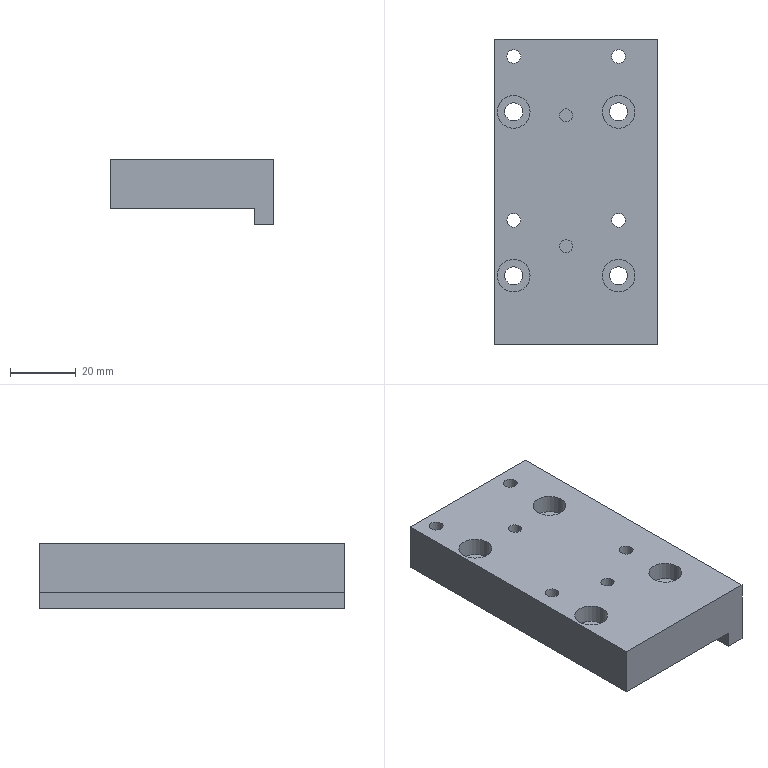Part | STEP file | SynoNew-0304-031 | 1 solid | 28 faces | box 50 x 93.3 x 20 mm | volume 69168 mm3 | cylinder 14 | plane 14 | commonest cylinder face diameters 4.2 x4 5.5 x4 10 x4 4 x2
STEP:
#1=CARTESIAN_POINT('',(-1.,-16.583,15.));
#2=VERTEX_POINT('',#1);
#3=CARTESIAN_POINT('',(-5.,-16.583,15.));
#4=VERTEX_POINT('',#3);
#5=CARTESIAN_POINT('',(-3.,-16.583,15.));
#6=DIRECTION('',(0.,0.,-1.));
#7=DIRECTION('',(1.,0.,0.));
#8=AXIS2_PLACEMENT_3D('',#5,#6,#7);
#9=CIRCLE('',#8,2.);
#10=EDGE_CURVE('',#2,#4,#9,.T.);
#11=ORIENTED_EDGE('',*,*,#10,.F.);
#12=CARTESIAN_POINT('',(-3.,-16.583,15.));
#13=DIRECTION('',(0.,0.,-1.));
#14=DIRECTION('',(1.,0.,0.));
#15=AXIS2_PLACEMENT_3D('',#12,#13,#14);
#16=CIRCLE('',#15,2.);
#17=EDGE_CURVE('',#4,#2,#16,.T.);
#18=ORIENTED_EDGE('',*,*,#17,.F.);
#19=CARTESIAN_POINT('',(-5.,-16.583,11.));
#20=VERTEX_POINT('',#19);
#21=CARTESIAN_POINT('',(-5.,-16.583,15.));
#22=DIRECTION('',(0.,0.,-1.));
#23=VECTOR('',#22,2.);
#24=LINE('',#21,#23);
#25=EDGE_CURVE('',#4,#20,#24,.T.);
#26=ORIENTED_EDGE('',*,*,#25,.T.);
#27=CARTESIAN_POINT('',(-1.,-16.583,11.));
#28=VERTEX_POINT('',#27);
#29=CARTESIAN_POINT('',(-3.,-16.583,11.));
#30=DIRECTION('',(0.,0.,-1.));
#31=DIRECTION('',(1.,0.,0.));
#32=AXIS2_PLACEMENT_3D('',#29,#30,#31);
#33=CIRCLE('',#32,2.);
#34=EDGE_CURVE('',#20,#28,#33,.T.);
#35=ORIENTED_EDGE('',*,*,#34,.T.);
#36=CARTESIAN_POINT('',(-3.,-16.583,11.));
#37=DIRECTION('',(0.,0.,-1.));
#38=DIRECTION('',(1.,0.,0.));
#39=AXIS2_PLACEMENT_3D('',#36,#37,#38);
#40=CIRCLE('',#39,2.);
#41=EDGE_CURVE('',#28,#20,#40,.T.);
#42=ORIENTED_EDGE('',*,*,#41,.T.);
#43=ORIENTED_EDGE('',*,*,#25,.F.);
#44=EDGE_LOOP('',(#11,#18,#26,#35,#42,#43));
#45=FACE_OUTER_BOUND('',#44,.T.);
#46=CARTESIAN_POINT('',(-3.,-16.583,15.));
#47=DIRECTION('',(0.,0.,-1.));
#48=DIRECTION('',(1.,0.,0.));
#49=AXIS2_PLACEMENT_3D('',#46,#47,#48);
#50=CYLINDRICAL_SURFACE('',#49,2.);
#51=ADVANCED_FACE('',(#45),#50,.F.);
#52=ORIENTED_EDGE('',*,*,#41,.F.);
#53=ORIENTED_EDGE('',*,*,#34,.F.);
#54=EDGE_LOOP('',(#52,#53));
#55=FACE_OUTER_BOUND('',#54,.T.);
#56=CARTESIAN_POINT('',(-3.,-16.583,11.));
#57=DIRECTION('',(0.,0.,1.));
#58=DIRECTION('',(1.,0.,0.));
#59=AXIS2_PLACEMENT_3D('',#56,#57,#58);
#60=PLANE('',#59);
#61=ADVANCED_FACE('',(#55),#60,.T.);
#62=CARTESIAN_POINT('',(-1.,23.35,15.));
#63=VERTEX_POINT('',#62);
#64=CARTESIAN_POINT('',(-5.,23.35,15.));
#65=VERTEX_POINT('',#64);
#66=CARTESIAN_POINT('',(-3.,23.35,15.));
#67=DIRECTION('',(0.,0.,-1.));
#68=DIRECTION('',(1.,0.,0.));
#69=AXIS2_PLACEMENT_3D('',#66,#67,#68);
#70=CIRCLE('',#69,2.);
#71=EDGE_CURVE('',#63,#65,#70,.T.);
#72=ORIENTED_EDGE('',*,*,#71,.F.);
#73=CARTESIAN_POINT('',(-3.,23.35,15.));
#74=DIRECTION('',(0.,0.,-1.));
#75=DIRECTION('',(1.,0.,0.));
#76=AXIS2_PLACEMENT_3D('',#73,#74,#75);
#77=CIRCLE('',#76,2.);
#78=EDGE_CURVE('',#65,#63,#77,.T.);
#79=ORIENTED_EDGE('',*,*,#78,.F.);
#80=CARTESIAN_POINT('',(-5.,23.35,11.));
#81=VERTEX_POINT('',#80);
#82=CARTESIAN_POINT('',(-5.,23.35,15.));
#83=DIRECTION('',(0.,0.,-1.));
#84=VECTOR('',#83,2.);
#85=LINE('',#82,#84);
#86=EDGE_CURVE('',#65,#81,#85,.T.);
#87=ORIENTED_EDGE('',*,*,#86,.T.);
#88=CARTESIAN_POINT('',(-1.,23.35,11.));
#89=VERTEX_POINT('',#88);
#90=CARTESIAN_POINT('',(-3.,23.35,11.));
#91=DIRECTION('',(0.,0.,-1.));
#92=DIRECTION('',(1.,0.,0.));
#93=AXIS2_PLACEMENT_3D('',#90,#91,#92);
#94=CIRCLE('',#93,2.);
#95=EDGE_CURVE('',#81,#89,#94,.T.);
#96=ORIENTED_EDGE('',*,*,#95,.T.);
#97=CARTESIAN_POINT('',(-3.,23.35,11.));
#98=DIRECTION('',(0.,0.,-1.));
#99=DIRECTION('',(1.,0.,0.));
#100=AXIS2_PLACEMENT_3D('',#97,#98,#99);
#101=CIRCLE('',#100,2.);
#102=EDGE_CURVE('',#89,#81,#101,.T.);
#103=ORIENTED_EDGE('',*,*,#102,.T.);
#104=ORIENTED_EDGE('',*,*,#86,.F.);
#105=EDGE_LOOP('',(#72,#79,#87,#96,#103,#104));
#106=FACE_OUTER_BOUND('',#105,.T.);
#107=CARTESIAN_POINT('',(-3.,23.35,15.));
#108=DIRECTION('',(0.,0.,-1.));
#109=DIRECTION('',(1.,0.,0.));
#110=AXIS2_PLACEMENT_3D('',#107,#108,#109);
#111=CYLINDRICAL_SURFACE('',#110,2.);
#112=ADVANCED_FACE('',(#106),#111,.F.);
#113=ORIENTED_EDGE('',*,*,#102,.F.);
#114=ORIENTED_EDGE('',*,*,#95,.F.);
#115=EDGE_LOOP('',(#113,#114));
#116=FACE_OUTER_BOUND('',#115,.T.);
#117=CARTESIAN_POINT('',(-3.,23.35,11.));
#118=DIRECTION('',(0.,0.,1.));
#119=DIRECTION('',(1.,0.,0.));
#120=AXIS2_PLACEMENT_3D('',#117,#118,#119);
#121=PLANE('',#120);
#122=ADVANCED_FACE('',(#116),#121,.T.);
#123=CARTESIAN_POINT('',(15.1,-8.65,15.));
#124=VERTEX_POINT('',#123);
#125=CARTESIAN_POINT('',(10.9,-8.65,15.));
#126=VERTEX_POINT('',#125);
#127=CARTESIAN_POINT('',(13.,-8.65,15.));
#128=DIRECTION('',(0.,0.,-1.));
#129=DIRECTION('',(1.,0.,0.));
#130=AXIS2_PLACEMENT_3D('',#127,#128,#129);
#131=CIRCLE('',#130,2.1);
#132=EDGE_CURVE('',#124,#126,#131,.T.);
#133=ORIENTED_EDGE('',*,*,#132,.F.);
#134=CARTESIAN_POINT('',(13.,-8.65,15.));
#135=DIRECTION('',(0.,0.,-1.));
#136=DIRECTION('',(1.,0.,0.));
#137=AXIS2_PLACEMENT_3D('',#134,#135,#136);
#138=CIRCLE('',#137,2.1);
#139=EDGE_CURVE('',#126,#124,#138,.T.);
#140=ORIENTED_EDGE('',*,*,#139,.F.);
#141=CARTESIAN_POINT('',(10.9,-8.65,0.));
#142=VERTEX_POINT('',#141);
#143=CARTESIAN_POINT('',(10.9,-8.65,-92.726));
#144=DIRECTION('',(0.,0.,-1.));
#145=VECTOR('',#144,2.1);
#146=LINE('',#143,#145);
#147=EDGE_CURVE('',#126,#142,#146,.T.);
#148=ORIENTED_EDGE('',*,*,#147,.T.);
#149=CARTESIAN_POINT('',(13.,-8.65,0.));
#150=DIRECTION('',(0.,0.,1.));
#151=DIRECTION('',(1.,0.,0.));
#152=AXIS2_PLACEMENT_3D('',#149,#150,#151);
#153=CIRCLE('',#152,2.1);
#154=EDGE_CURVE('',#142,#142,#153,.T.);
#155=ORIENTED_EDGE('',*,*,#154,.F.);
#156=ORIENTED_EDGE('',*,*,#147,.F.);
#157=EDGE_LOOP('',(#133,#140,#148,#155,#156));
#158=FACE_OUTER_BOUND('',#157,.T.);
#159=CARTESIAN_POINT('',(13.,-8.65,-92.726));
#160=DIRECTION('',(0.,0.,1.));
#161=DIRECTION('',(1.,0.,0.));
#162=AXIS2_PLACEMENT_3D('',#159,#160,#161);
#163=CYLINDRICAL_SURFACE('',#162,2.1);
#164=ADVANCED_FACE('',(#158),#163,.F.);
#165=CARTESIAN_POINT('',(-16.9,41.35,15.));
#166=VERTEX_POINT('',#165);
#167=CARTESIAN_POINT('',(-21.1,41.35,15.));
#168=VERTEX_POINT('',#167);
#169=CARTESIAN_POINT('',(-19.,41.35,15.));
#170=DIRECTION('',(0.,0.,-1.));
#171=DIRECTION('',(1.,0.,0.));
#172=AXIS2_PLACEMENT_3D('',#169,#170,#171);
#173=CIRCLE('',#172,2.1);
#174=EDGE_CURVE('',#166,#168,#173,.T.);
#175=ORIENTED_EDGE('',*,*,#174,.F.);
#176=CARTESIAN_POINT('',(-19.,41.35,15.));
#177=DIRECTION('',(0.,0.,-1.));
#178=DIRECTION('',(1.,0.,0.));
#179=AXIS2_PLACEMENT_3D('',#176,#177,#178);
#180=CIRCLE('',#179,2.1);
#181=EDGE_CURVE('',#168,#166,#180,.T.);
#182=ORIENTED_EDGE('',*,*,#181,.F.);
#183=CARTESIAN_POINT('',(-21.1,41.35,0.));
#184=VERTEX_POINT('',#183);
#185=CARTESIAN_POINT('',(-21.1,41.35,-92.726));
#186=DIRECTION('',(0.,0.,-1.));
#187=VECTOR('',#186,2.1);
#188=LINE('',#185,#187);
#189=EDGE_CURVE('',#168,#184,#188,.T.);
#190=ORIENTED_EDGE('',*,*,#189,.T.);
#191=CARTESIAN_POINT('',(-19.,41.35,0.));
#192=DIRECTION('',(0.,0.,1.));
#193=DIRECTION('',(1.,0.,0.));
#194=AXIS2_PLACEMENT_3D('',#191,#192,#193);
#195=CIRCLE('',#194,2.1);
#196=EDGE_CURVE('',#184,#184,#195,.T.);
#197=ORIENTED_EDGE('',*,*,#196,.F.);
#198=ORIENTED_EDGE('',*,*,#189,.F.);
#199=EDGE_LOOP('',(#175,#182,#190,#197,#198));
#200=FACE_OUTER_BOUND('',#199,.T.);
#201=CARTESIAN_POINT('',(-19.,41.35,-92.726));
#202=DIRECTION('',(0.,0.,1.));
#203=DIRECTION('',(1.,0.,0.));
#204=AXIS2_PLACEMENT_3D('',#201,#202,#203);
#205=CYLINDRICAL_SURFACE('',#204,2.1);
#206=ADVANCED_FACE('',(#200),#205,.F.);
#207=CARTESIAN_POINT('',(15.1,41.35,15.));
#208=VERTEX_POINT('',#207);
#209=CARTESIAN_POINT('',(10.9,41.35,15.));
#210=VERTEX_POINT('',#209);
#211=CARTESIAN_POINT('',(13.,41.35,15.));
#212=DIRECTION('',(0.,0.,-1.));
#213=DIRECTION('',(1.,0.,0.));
#214=AXIS2_PLACEMENT_3D('',#211,#212,#213);
#215=CIRCLE('',#214,2.1);
#216=EDGE_CURVE('',#208,#210,#215,.T.);
#217=ORIENTED_EDGE('',*,*,#216,.F.);
#218=CARTESIAN_POINT('',(13.,41.35,15.));
#219=DIRECTION('',(0.,0.,-1.));
#220=DIRECTION('',(1.,0.,0.));
#221=AXIS2_PLACEMENT_3D('',#218,#219,#220);
#222=CIRCLE('',#221,2.1);
#223=EDGE_CURVE('',#210,#208,#222,.T.);
#224=ORIENTED_EDGE('',*,*,#223,.F.);
#225=CARTESIAN_POINT('',(10.9,41.35,0.));
#226=VERTEX_POINT('',#225);
#227=CARTESIAN_POINT('',(10.9,41.35,-92.726));
#228=DIRECTION('',(0.,0.,-1.));
#229=VECTOR('',#228,2.1);
#230=LINE('',#227,#229);
#231=EDGE_CURVE('',#210,#226,#230,.T.);
#232=ORIENTED_EDGE('',*,*,#231,.T.);
#233=CARTESIAN_POINT('',(13.,41.35,0.));
#234=DIRECTION('',(0.,0.,1.));
#235=DIRECTION('',(1.,0.,0.));
#236=AXIS2_PLACEMENT_3D('',#233,#234,#235);
#237=CIRCLE('',#236,2.1);
#238=EDGE_CURVE('',#226,#226,#237,.T.);
#239=ORIENTED_EDGE('',*,*,#238,.F.);
#240=ORIENTED_EDGE('',*,*,#231,.F.);
#241=EDGE_LOOP('',(#217,#224,#232,#239,#240));
#242=FACE_OUTER_BOUND('',#241,.T.);
#243=CARTESIAN_POINT('',(13.,41.35,-92.726));
#244=DIRECTION('',(0.,0.,1.));
#245=DIRECTION('',(1.,0.,0.));
#246=AXIS2_PLACEMENT_3D('',#243,#244,#245);
#247=CYLINDRICAL_SURFACE('',#246,2.1);
#248=ADVANCED_FACE('',(#242),#247,.F.);
#249=CARTESIAN_POINT('',(-16.9,-8.65,15.));
#250=VERTEX_POINT('',#249);
#251=CARTESIAN_POINT('',(-21.1,-8.65,15.));
#252=VERTEX_POINT('',#251);
#253=CARTESIAN_POINT('',(-19.,-8.65,15.));
#254=DIRECTION('',(0.,0.,-1.));
#255=DIRECTION('',(1.,0.,0.));
#256=AXIS2_PLACEMENT_3D('',#253,#254,#255);
#257=CIRCLE('',#256,2.1);
#258=EDGE_CURVE('',#250,#252,#257,.T.);
#259=ORIENTED_EDGE('',*,*,#258,.F.);
#260=CARTESIAN_POINT('',(-19.,-8.65,15.));
#261=DIRECTION('',(0.,0.,-1.));
#262=DIRECTION('',(1.,0.,0.));
#263=AXIS2_PLACEMENT_3D('',#260,#261,#262);
#264=CIRCLE('',#263,2.1);
#265=EDGE_CURVE('',#252,#250,#264,.T.);
#266=ORIENTED_EDGE('',*,*,#265,.F.);
#267=CARTESIAN_POINT('',(-21.1,-8.65,0.));
#268=VERTEX_POINT('',#267);
#269=CARTESIAN_POINT('',(-21.1,-8.65,-92.726));
#270=DIRECTION('',(0.,0.,-1.));
#271=VECTOR('',#270,2.1);
#272=LINE('',#269,#271);
#273=EDGE_CURVE('',#252,#268,#272,.T.);
#274=ORIENTED_EDGE('',*,*,#273,.T.);
#275=CARTESIAN_POINT('',(-19.,-8.65,0.));
#276=DIRECTION('',(0.,0.,1.));
#277=DIRECTION('',(1.,0.,0.));
#278=AXIS2_PLACEMENT_3D('',#275,#276,#277);
#279=CIRCLE('',#278,2.1);
#280=EDGE_CURVE('',#268,#268,#279,.T.);
#281=ORIENTED_EDGE('',*,*,#280,.F.);
#282=ORIENTED_EDGE('',*,*,#273,.F.);
#283=EDGE_LOOP('',(#259,#266,#274,#281,#282));
#284=FACE_OUTER_BOUND('',#283,.T.);
#285=CARTESIAN_POINT('',(-19.,-8.65,-92.726));
#286=DIRECTION('',(0.,0.,1.));
#287=DIRECTION('',(1.,0.,0.));
#288=AXIS2_PLACEMENT_3D('',#285,#286,#287);
#289=CYLINDRICAL_SURFACE('',#288,2.1);
#290=ADVANCED_FACE('',(#284),#289,.F.);
#291=CARTESIAN_POINT('',(18.,-25.55,9.3));
#292=VERTEX_POINT('',#291);
#293=CARTESIAN_POINT('',(8.,-25.55,9.3));
#294=VERTEX_POINT('',#293);
#295=CARTESIAN_POINT('',(13.,-25.55,9.3));
#296=DIRECTION('',(0.,0.,1.));
#297=DIRECTION('',(1.,0.,0.));
#298=AXIS2_PLACEMENT_3D('',#295,#296,#297);
#299=CIRCLE('',#298,5.);
#300=EDGE_CURVE('',#292,#294,#299,.T.);
#301=ORIENTED_EDGE('',*,*,#300,.T.);
#302=CARTESIAN_POINT('',(13.,-25.55,9.3));
#303=DIRECTION('',(0.,0.,1.));
#304=DIRECTION('',(1.,0.,0.));
#305=AXIS2_PLACEMENT_3D('',#302,#303,#304);
#306=CIRCLE('',#305,5.);
#307=EDGE_CURVE('',#294,#292,#306,.T.);
#308=ORIENTED_EDGE('',*,*,#307,.T.);
#309=EDGE_LOOP('',(#301,#308));
#310=FACE_OUTER_BOUND('',#309,.T.);
#311=CARTESIAN_POINT('',(10.25,-25.55,9.3));
#312=VERTEX_POINT('',#311);
#313=CARTESIAN_POINT('',(13.,-25.55,9.3));
#314=DIRECTION('',(0.,0.,1.));
#315=DIRECTION('',(1.,0.,0.));
#316=AXIS2_PLACEMENT_3D('',#313,#314,#315);
#317=CIRCLE('',#316,2.75);
#318=EDGE_CURVE('',#312,#312,#317,.T.);
#319=ORIENTED_EDGE('',*,*,#318,.F.);
#320=EDGE_LOOP('',(#319));
#321=FACE_BOUND('',#320,.T.);
#322=CARTESIAN_POINT('',(13.,-25.55,9.3));
#323=DIRECTION('',(0.,0.,1.));
#324=DIRECTION('',(1.,0.,0.));
#325=AXIS2_PLACEMENT_3D('',#322,#323,#324);
#326=PLANE('',#325);
#327=ADVANCED_FACE('',(#310,#321),#326,.T.);
#328=CARTESIAN_POINT('',(18.,-25.55,15.));
#329=VERTEX_POINT('',#328);
#330=CARTESIAN_POINT('',(8.,-25.55,15.));
#331=VERTEX_POINT('',#330);
#332=CARTESIAN_POINT('',(13.,-25.55,15.));
#333=DIRECTION('',(0.,0.,-1.));
#334=DIRECTION('',(1.,0.,0.));
#335=AXIS2_PLACEMENT_3D('',#332,#333,#334);
#336=CIRCLE('',#335,5.);
#337=EDGE_CURVE('',#329,#331,#336,.T.);
#338=ORIENTED_EDGE('',*,*,#337,.F.);
#339=CARTESIAN_POINT('',(13.,-25.55,15.));
#340=DIRECTION('',(0.,0.,-1.));
#341=DIRECTION('',(1.,0.,0.));
#342=AXIS2_PLACEMENT_3D('',#339,#340,#341);
#343=CIRCLE('',#342,5.);
#344=EDGE_CURVE('',#331,#329,#343,.T.);
#345=ORIENTED_EDGE('',*,*,#344,.F.);
#346=CARTESIAN_POINT('',(8.,-25.55,12.15));
#347=DIRECTION('',(0.,0.,-1.));
#348=VECTOR('',#347,5.);
#349=LINE('',#346,#348);
#350=EDGE_CURVE('',#331,#294,#349,.T.);
#351=ORIENTED_EDGE('',*,*,#350,.T.);
#352=ORIENTED_EDGE('',*,*,#300,.F.);
#353=ORIENTED_EDGE('',*,*,#307,.F.);
#354=ORIENTED_EDGE('',*,*,#350,.F.);
#355=EDGE_LOOP('',(#338,#345,#351,#352,#353,#354));
#356=FACE_OUTER_BOUND('',#355,.T.);
#357=CARTESIAN_POINT('',(13.,-25.55,12.15));
#358=DIRECTION('',(0.,0.,1.));
#359=DIRECTION('',(1.,0.,0.));
#360=AXIS2_PLACEMENT_3D('',#357,#358,#359);
#361=CYLINDRICAL_SURFACE('',#360,5.);
#362=ADVANCED_FACE('',(#356),#361,.F.);
#363=ORIENTED_EDGE('',*,*,#318,.T.);
#364=CARTESIAN_POINT('',(10.25,-25.55,0.));
#365=VERTEX_POINT('',#364);
#366=CARTESIAN_POINT('',(10.25,-25.55,-92.726));
#367=DIRECTION('',(0.,0.,-1.));
#368=VECTOR('',#367,2.75);
#369=LINE('',#366,#368);
#370=EDGE_CURVE('',#312,#365,#369,.T.);
#371=ORIENTED_EDGE('',*,*,#370,.T.);
#372=CARTESIAN_POINT('',(13.,-25.55,0.));
#373=DIRECTION('',(0.,0.,1.));
#374=DIRECTION('',(1.,0.,0.));
#375=AXIS2_PLACEMENT_3D('',#372,#373,#374);
#376=CIRCLE('',#375,2.75);
#377=EDGE_CURVE('',#365,#365,#376,.T.);
#378=ORIENTED_EDGE('',*,*,#377,.F.);
#379=ORIENTED_EDGE('',*,*,#370,.F.);
#380=EDGE_LOOP('',(#363,#371,#378,#379));
#381=FACE_OUTER_BOUND('',#380,.T.);
#382=CARTESIAN_POINT('',(13.,-25.55,-92.726));
#383=DIRECTION('',(0.,0.,1.));
#384=DIRECTION('',(1.,0.,0.));
#385=AXIS2_PLACEMENT_3D('',#382,#383,#384);
#386=CYLINDRICAL_SURFACE('',#385,2.75);
#387=ADVANCED_FACE('',(#381),#386,.F.);
#388=CARTESIAN_POINT('',(18.,24.45,9.3));
#389=VERTEX_POINT('',#388);
#390=CARTESIAN_POINT('',(8.,24.45,9.3));
#391=VERTEX_POINT('',#390);
#392=CARTESIAN_POINT('',(13.,24.45,9.3));
#393=DIRECTION('',(0.,0.,1.));
#394=DIRECTION('',(1.,0.,0.));
#395=AXIS2_PLACEMENT_3D('',#392,#393,#394);
#396=CIRCLE('',#395,5.);
#397=EDGE_CURVE('',#389,#391,#396,.T.);
#398=ORIENTED_EDGE('',*,*,#397,.T.);
#399=CARTESIAN_POINT('',(13.,24.45,9.3));
#400=DIRECTION('',(0.,0.,1.));
#401=DIRECTION('',(1.,0.,0.));
#402=AXIS2_PLACEMENT_3D('',#399,#400,#401);
#403=CIRCLE('',#402,5.);
#404=EDGE_CURVE('',#391,#389,#403,.T.);
#405=ORIENTED_EDGE('',*,*,#404,.T.);
#406=EDGE_LOOP('',(#398,#405));
#407=FACE_OUTER_BOUND('',#406,.T.);
#408=CARTESIAN_POINT('',(10.25,24.45,9.3));
#409=VERTEX_POINT('',#408);
#410=CARTESIAN_POINT('',(13.,24.45,9.3));
#411=DIRECTION('',(0.,0.,1.));
#412=DIRECTION('',(1.,0.,0.));
#413=AXIS2_PLACEMENT_3D('',#410,#411,#412);
#414=CIRCLE('',#413,2.75);
#415=EDGE_CURVE('',#409,#409,#414,.T.);
#416=ORIENTED_EDGE('',*,*,#415,.F.);
#417=EDGE_LOOP('',(#416));
#418=FACE_BOUND('',#417,.T.);
#419=CARTESIAN_POINT('',(13.,24.45,9.3));
#420=DIRECTION('',(0.,0.,1.));
#421=DIRECTION('',(1.,0.,0.));
#422=AXIS2_PLACEMENT_3D('',#419,#420,#421);
#423=PLANE('',#422);
#424=ADVANCED_FACE('',(#407,#418),#423,.T.);
#425=CARTESIAN_POINT('',(18.,24.45,15.));
#426=VERTEX_POINT('',#425);
#427=CARTESIAN_POINT('',(8.,24.45,15.));
#428=VERTEX_POINT('',#427);
#429=CARTESIAN_POINT('',(13.,24.45,15.));
#430=DIRECTION('',(0.,0.,-1.));
#431=DIRECTION('',(1.,0.,0.));
#432=AXIS2_PLACEMENT_3D('',#429,#430,#431);
#433=CIRCLE('',#432,5.);
#434=EDGE_CURVE('',#426,#428,#433,.T.);
#435=ORIENTED_EDGE('',*,*,#434,.F.);
#436=CARTESIAN_POINT('',(13.,24.45,15.));
#437=DIRECTION('',(0.,0.,-1.));
#438=DIRECTION('',(1.,0.,0.));
#439=AXIS2_PLACEMENT_3D('',#436,#437,#438);
#440=CIRCLE('',#439,5.);
#441=EDGE_CURVE('',#428,#426,#440,.T.);
#442=ORIENTED_EDGE('',*,*,#441,.F.);
#443=CARTESIAN_POINT('',(8.,24.45,12.15));
#444=DIRECTION('',(0.,0.,-1.));
#445=VECTOR('',#444,5.);
#446=LINE('',#443,#445);
#447=EDGE_CURVE('',#428,#391,#446,.T.);
#448=ORIENTED_EDGE('',*,*,#447,.T.);
#449=ORIENTED_EDGE('',*,*,#397,.F.);
#450=ORIENTED_EDGE('',*,*,#404,.F.);
#451=ORIENTED_EDGE('',*,*,#447,.F.);
#452=EDGE_LOOP('',(#435,#442,#448,#449,#450,#451));
#453=FACE_OUTER_BOUND('',#452,.T.);
#454=CARTESIAN_POINT('',(13.,24.45,12.15));
#455=DIRECTION('',(0.,0.,1.));
#456=DIRECTION('',(1.,0.,0.));
#457=AXIS2_PLACEMENT_3D('',#454,#455,#456);
#458=CYLINDRICAL_SURFACE('',#457,5.);
#459=ADVANCED_FACE('',(#453),#458,.F.);
#460=ORIENTED_EDGE('',*,*,#415,.T.);
#461=CARTESIAN_POINT('',(10.25,24.45,0.));
#462=VERTEX_POINT('',#461);
#463=CARTESIAN_POINT('',(10.25,24.45,-92.726));
#464=DIRECTION('',(0.,0.,-1.));
#465=VECTOR('',#464,2.75);
#466=LINE('',#463,#465);
#467=EDGE_CURVE('',#409,#462,#466,.T.);
#468=ORIENTED_EDGE('',*,*,#467,.T.);
#469=CARTESIAN_POINT('',(13.,24.45,0.));
#470=DIRECTION('',(0.,0.,1.));
#471=DIRECTION('',(1.,0.,0.));
#472=AXIS2_PLACEMENT_3D('',#469,#470,#471);
#473=CIRCLE('',#472,2.75);
#474=EDGE_CURVE('',#462,#462,#473,.T.);
#475=ORIENTED_EDGE('',*,*,#474,.F.);
#476=ORIENTED_EDGE('',*,*,#467,.F.);
#477=EDGE_LOOP('',(#460,#468,#475,#476));
#478=FACE_OUTER_BOUND('',#477,.T.);
#479=CARTESIAN_POINT('',(13.,24.45,-92.726));
#480=DIRECTION('',(0.,0.,1.));
#481=DIRECTION('',(1.,0.,0.));
#482=AXIS2_PLACEMENT_3D('',#479,#480,#481);
#483=CYLINDRICAL_SURFACE('',#482,2.75);
#484=ADVANCED_FACE('',(#478),#483,.F.);
#485=CARTESIAN_POINT('',(-14.,24.45,9.3));
#486=VERTEX_POINT('',#485);
#487=CARTESIAN_POINT('',(-24.,24.45,9.3));
#488=VERTEX_POINT('',#487);
#489=CARTESIAN_POINT('',(-19.,24.45,9.3));
#490=DIRECTION('',(0.,0.,1.));
#491=DIRECTION('',(1.,0.,0.));
#492=AXIS2_PLACEMENT_3D('',#489,#490,#491);
#493=CIRCLE('',#492,5.);
#494=EDGE_CURVE('',#486,#488,#493,.T.);
#495=ORIENTED_EDGE('',*,*,#494,.T.);
#496=CARTESIAN_POINT('',(-19.,24.45,9.3));
#497=DIRECTION('',(0.,0.,1.));
#498=DIRECTION('',(1.,0.,0.));
#499=AXIS2_PLACEMENT_3D('',#496,#497,#498);
#500=CIRCLE('',#499,5.);
#501=EDGE_CURVE('',#488,#486,#500,.T.);
#502=ORIENTED_EDGE('',*,*,#501,.T.);
#503=EDGE_LOOP('',(#495,#502));
#504=FACE_OUTER_BOUND('',#503,.T.);
#505=CARTESIAN_POINT('',(-21.75,24.45,9.3));
#506=VERTEX_POINT('',#505);
#507=CARTESIAN_POINT('',(-19.,24.45,9.3));
#508=DIRECTION('',(0.,0.,1.));
#509=DIRECTION('',(1.,0.,0.));
#510=AXIS2_PLACEMENT_3D('',#507,#508,#509);
#511=CIRCLE('',#510,2.75);
#512=EDGE_CURVE('',#506,#506,#511,.T.);
#513=ORIENTED_EDGE('',*,*,#512,.F.);
#514=EDGE_LOOP('',(#513));
#515=FACE_BOUND('',#514,.T.);
#516=CARTESIAN_POINT('',(-19.,24.45,9.3));
#517=DIRECTION('',(0.,0.,1.));
#518=DIRECTION('',(1.,0.,0.));
#519=AXIS2_PLACEMENT_3D('',#516,#517,#518);
#520=PLANE('',#519);
#521=ADVANCED_FACE('',(#504,#515),#520,.T.);
#522=CARTESIAN_POINT('',(-14.,24.45,15.));
#523=VERTEX_POINT('',#522);
#524=CARTESIAN_POINT('',(-24.,24.45,15.));
#525=VERTEX_POINT('',#524);
#526=CARTESIAN_POINT('',(-19.,24.45,15.));
#527=DIRECTION('',(0.,0.,-1.));
#528=DIRECTION('',(1.,0.,0.));
#529=AXIS2_PLACEMENT_3D('',#526,#527,#528);
#530=CIRCLE('',#529,5.);
#531=EDGE_CURVE('',#523,#525,#530,.T.);
#532=ORIENTED_EDGE('',*,*,#531,.F.);
#533=CARTESIAN_POINT('',(-19.,24.45,15.));
#534=DIRECTION('',(0.,0.,-1.));
#535=DIRECTION('',(1.,0.,0.));
#536=AXIS2_PLACEMENT_3D('',#533,#534,#535);
#537=CIRCLE('',#536,5.);
#538=EDGE_CURVE('',#525,#523,#537,.T.);
#539=ORIENTED_EDGE('',*,*,#538,.F.);
#540=CARTESIAN_POINT('',(-24.,24.45,12.15));
#541=DIRECTION('',(0.,0.,-1.));
#542=VECTOR('',#541,5.);
#543=LINE('',#540,#542);
#544=EDGE_CURVE('',#525,#488,#543,.T.);
#545=ORIENTED_EDGE('',*,*,#544,.T.);
#546=ORIENTED_EDGE('',*,*,#494,.F.);
#547=ORIENTED_EDGE('',*,*,#501,.F.);
#548=ORIENTED_EDGE('',*,*,#544,.F.);
#549=EDGE_LOOP('',(#532,#539,#545,#546,#547,#548));
#550=FACE_OUTER_BOUND('',#549,.T.);
#551=CARTESIAN_POINT('',(-19.,24.45,12.15));
#552=DIRECTION('',(0.,0.,1.));
#553=DIRECTION('',(1.,0.,0.));
#554=AXIS2_PLACEMENT_3D('',#551,#552,#553);
#555=CYLINDRICAL_SURFACE('',#554,5.);
#556=ADVANCED_FACE('',(#550),#555,.F.);
#557=ORIENTED_EDGE('',*,*,#512,.T.);
#558=CARTESIAN_POINT('',(-21.75,24.45,0.));
#559=VERTEX_POINT('',#558);
#560=CARTESIAN_POINT('',(-21.75,24.45,-92.726));
#561=DIRECTION('',(0.,0.,-1.));
#562=VECTOR('',#561,2.75);
#563=LINE('',#560,#562);
#564=EDGE_CURVE('',#506,#559,#563,.T.);
#565=ORIENTED_EDGE('',*,*,#564,.T.);
#566=CARTESIAN_POINT('',(-19.,24.45,0.));
#567=DIRECTION('',(0.,0.,1.));
#568=DIRECTION('',(1.,0.,0.));
#569=AXIS2_PLACEMENT_3D('',#566,#567,#568);
#570=CIRCLE('',#569,2.75);
#571=EDGE_CURVE('',#559,#559,#570,.T.);
#572=ORIENTED_EDGE('',*,*,#571,.F.);
#573=ORIENTED_EDGE('',*,*,#564,.F.);
#574=EDGE_LOOP('',(#557,#565,#572,#573));
#575=FACE_OUTER_BOUND('',#574,.T.);
#576=CARTESIAN_POINT('',(-19.,24.45,-92.726));
#577=DIRECTION('',(0.,0.,1.));
#578=DIRECTION('',(1.,0.,0.));
#579=AXIS2_PLACEMENT_3D('',#576,#577,#578);
#580=CYLINDRICAL_SURFACE('',#579,2.75);
#581=ADVANCED_FACE('',(#575),#580,.F.);
#582=CARTESIAN_POINT('',(-14.,-25.55,9.3));
#583=VERTEX_POINT('',#582);
#584=CARTESIAN_POINT('',(-24.,-25.55,9.3));
#585=VERTEX_POINT('',#584);
#586=CARTESIAN_POINT('',(-19.,-25.55,9.3));
#587=DIRECTION('',(0.,0.,1.));
#588=DIRECTION('',(1.,0.,0.));
#589=AXIS2_PLACEMENT_3D('',#586,#587,#588);
#590=CIRCLE('',#589,5.);
#591=EDGE_CURVE('',#583,#585,#590,.T.);
#592=ORIENTED_EDGE('',*,*,#591,.T.);
#593=CARTESIAN_POINT('',(-19.,-25.55,9.3));
#594=DIRECTION('',(0.,0.,1.));
#595=DIRECTION('',(1.,0.,0.));
#596=AXIS2_PLACEMENT_3D('',#593,#594,#595);
#597=CIRCLE('',#596,5.);
#598=EDGE_CURVE('',#585,#583,#597,.T.);
#599=ORIENTED_EDGE('',*,*,#598,.T.);
#600=EDGE_LOOP('',(#592,#599));
#601=FACE_OUTER_BOUND('',#600,.T.);
#602=CARTESIAN_POINT('',(-21.75,-25.55,9.3));
#603=VERTEX_POINT('',#602);
#604=CARTESIAN_POINT('',(-19.,-25.55,9.3));
#605=DIRECTION('',(0.,0.,1.));
#606=DIRECTION('',(1.,0.,0.));
#607=AXIS2_PLACEMENT_3D('',#604,#605,#606);
#608=CIRCLE('',#607,2.75);
#609=EDGE_CURVE('',#603,#603,#608,.T.);
#610=ORIENTED_EDGE('',*,*,#609,.F.);
#611=EDGE_LOOP('',(#610));
#612=FACE_BOUND('',#611,.T.);
#613=CARTESIAN_POINT('',(-19.,-25.55,9.3));
#614=DIRECTION('',(0.,0.,1.));
#615=DIRECTION('',(1.,0.,0.));
#616=AXIS2_PLACEMENT_3D('',#613,#614,#615);
#617=PLANE('',#616);
#618=ADVANCED_FACE('',(#601,#612),#617,.T.);
#619=CARTESIAN_POINT('',(-14.,-25.55,15.));
#620=VERTEX_POINT('',#619);
#621=CARTESIAN_POINT('',(-24.,-25.55,15.));
#622=VERTEX_POINT('',#621);
#623=CARTESIAN_POINT('',(-19.,-25.55,15.));
#624=DIRECTION('',(0.,0.,-1.));
#625=DIRECTION('',(1.,0.,0.));
#626=AXIS2_PLACEMENT_3D('',#623,#624,#625);
#627=CIRCLE('',#626,5.);
#628=EDGE_CURVE('',#620,#622,#627,.T.);
#629=ORIENTED_EDGE('',*,*,#628,.F.);
#630=CARTESIAN_POINT('',(-19.,-25.55,15.));
#631=DIRECTION('',(0.,0.,-1.));
#632=DIRECTION('',(1.,0.,0.));
#633=AXIS2_PLACEMENT_3D('',#630,#631,#632);
#634=CIRCLE('',#633,5.);
#635=EDGE_CURVE('',#622,#620,#634,.T.);
#636=ORIENTED_EDGE('',*,*,#635,.F.);
#637=CARTESIAN_POINT('',(-24.,-25.55,12.15));
#638=DIRECTION('',(0.,0.,-1.));
#639=VECTOR('',#638,5.);
#640=LINE('',#637,#639);
#641=EDGE_CURVE('',#622,#585,#640,.T.);
#642=ORIENTED_EDGE('',*,*,#641,.T.);
#643=ORIENTED_EDGE('',*,*,#591,.F.);
#644=ORIENTED_EDGE('',*,*,#598,.F.);
#645=ORIENTED_EDGE('',*,*,#641,.F.);
#646=EDGE_LOOP('',(#629,#636,#642,#643,#644,#645));
#647=FACE_OUTER_BOUND('',#646,.T.);
#648=CARTESIAN_POINT('',(-19.,-25.55,12.15));
#649=DIRECTION('',(0.,0.,1.));
#650=DIRECTION('',(1.,0.,0.));
#651=AXIS2_PLACEMENT_3D('',#648,#649,#650);
#652=CYLINDRICAL_SURFACE('',#651,5.);
#653=ADVANCED_FACE('',(#647),#652,.F.);
#654=ORIENTED_EDGE('',*,*,#609,.T.);
#655=CARTESIAN_POINT('',(-21.75,-25.55,0.));
#656=VERTEX_POINT('',#655);
#657=CARTESIAN_POINT('',(-21.75,-25.55,-92.726));
#658=DIRECTION('',(0.,0.,-1.));
#659=VECTOR('',#658,2.75);
#660=LINE('',#657,#659);
#661=EDGE_CURVE('',#603,#656,#660,.T.);
#662=ORIENTED_EDGE('',*,*,#661,.T.);
#663=CARTESIAN_POINT('',(-19.,-25.55,0.));
#664=DIRECTION('',(0.,0.,1.));
#665=DIRECTION('',(1.,0.,0.));
#666=AXIS2_PLACEMENT_3D('',#663,#664,#665);
#667=CIRCLE('',#666,2.75);
#668=EDGE_CURVE('',#656,#656,#667,.T.);
#669=ORIENTED_EDGE('',*,*,#668,.F.);
#670=ORIENTED_EDGE('',*,*,#661,.F.);
#671=EDGE_LOOP('',(#654,#662,#669,#670));
#672=FACE_OUTER_BOUND('',#671,.T.);
#673=CARTESIAN_POINT('',(-19.,-25.55,-92.726));
#674=DIRECTION('',(0.,0.,1.));
#675=DIRECTION('',(1.,0.,0.));
#676=AXIS2_PLACEMENT_3D('',#673,#674,#675);
#677=CYLINDRICAL_SURFACE('',#676,2.75);
#678=ADVANCED_FACE('',(#672),#677,.F.);
#679=CARTESIAN_POINT('',(19.,46.65,0.));
#680=VERTEX_POINT('',#679);
#681=CARTESIAN_POINT('',(19.,-46.65,0.));
#682=VERTEX_POINT('',#681);
#683=CARTESIAN_POINT('',(19.,-23.325,0.));
#684=DIRECTION('',(0.,-1.,0.));
#685=VECTOR('',#684,10.);
#686=LINE('',#683,#685);
#687=EDGE_CURVE('',#680,#682,#686,.T.);
#688=ORIENTED_EDGE('',*,*,#687,.F.);
#689=CARTESIAN_POINT('',(19.,46.65,-5.));
#690=VERTEX_POINT('',#689);
#691=CARTESIAN_POINT('',(19.,46.65,0.));
#692=DIRECTION('',(0.,0.,-1.));
#693=VECTOR('',#692,10.);
#694=LINE('',#691,#693);
#695=EDGE_CURVE('',#680,#690,#694,.T.);
#696=ORIENTED_EDGE('',*,*,#695,.T.);
#697=CARTESIAN_POINT('',(19.,-46.65,-5.));
#698=VERTEX_POINT('',#697);
#699=CARTESIAN_POINT('',(19.,-46.65,-5.));
#700=DIRECTION('',(0.,1.,0.));
#701=VECTOR('',#700,10.);
#702=LINE('',#699,#701);
#703=EDGE_CURVE('',#698,#690,#702,.T.);
#704=ORIENTED_EDGE('',*,*,#703,.F.);
#705=CARTESIAN_POINT('',(19.,-46.65,0.));
#706=DIRECTION('',(0.,0.,-1.));
#707=VECTOR('',#706,10.);
#708=LINE('',#705,#707);
#709=EDGE_CURVE('',#682,#698,#708,.T.);
#710=ORIENTED_EDGE('',*,*,#709,.F.);
#711=EDGE_LOOP('',(#688,#696,#704,#710));
#712=FACE_OUTER_BOUND('',#711,.T.);
#713=CARTESIAN_POINT('',(19.,-46.65,0.));
#714=DIRECTION('',(-1.,0.,0.));
#715=DIRECTION('',(0.,1.,0.));
#716=AXIS2_PLACEMENT_3D('',#713,#714,#715);
#717=PLANE('',#716);
#718=ADVANCED_FACE('',(#712),#717,.T.);
#719=CARTESIAN_POINT('',(25.,-46.65,-5.));
#720=VERTEX_POINT('',#719);
#721=CARTESIAN_POINT('',(25.,-46.65,-5.));
#722=DIRECTION('',(-1.,0.,0.));
#723=VECTOR('',#722,10.);
#724=LINE('',#721,#723);
#725=EDGE_CURVE('',#720,#698,#724,.T.);
#726=ORIENTED_EDGE('',*,*,#725,.T.);
#727=ORIENTED_EDGE('',*,*,#703,.T.);
#728=CARTESIAN_POINT('',(25.,46.65,-5.));
#729=VERTEX_POINT('',#728);
#730=CARTESIAN_POINT('',(-25.,46.65,-5.));
#731=DIRECTION('',(1.,0.,0.));
#732=VECTOR('',#731,10.);
#733=LINE('',#730,#732);
#734=EDGE_CURVE('',#690,#729,#733,.T.);
#735=ORIENTED_EDGE('',*,*,#734,.T.);
#736=CARTESIAN_POINT('',(25.,46.65,-5.));
#737=DIRECTION('',(0.,-1.,0.));
#738=VECTOR('',#737,10.);
#739=LINE('',#736,#738);
#740=EDGE_CURVE('',#729,#720,#739,.T.);
#741=ORIENTED_EDGE('',*,*,#740,.T.);
#742=EDGE_LOOP('',(#726,#727,#735,#741));
#743=FACE_OUTER_BOUND('',#742,.T.);
#744=CARTESIAN_POINT('',(22.,0.,-5.));
#745=DIRECTION('',(0.,0.,-1.));
#746=DIRECTION('',(-1.,0.,0.));
#747=AXIS2_PLACEMENT_3D('',#744,#745,#746);
#748=PLANE('',#747);
#749=ADVANCED_FACE('',(#743),#748,.T.);
#750=ORIENTED_EDGE('',*,*,#687,.T.);
#751=CARTESIAN_POINT('',(-25.,-46.65,0.));
#752=VERTEX_POINT('',#751);
#753=CARTESIAN_POINT('',(-25.,-46.65,0.));
#754=DIRECTION('',(1.,0.,0.));
#755=VECTOR('',#754,10.);
#756=LINE('',#753,#755);
#757=EDGE_CURVE('',#752,#682,#756,.T.);
#758=ORIENTED_EDGE('',*,*,#757,.F.);
#759=CARTESIAN_POINT('',(-25.,46.65,0.));
#760=VERTEX_POINT('',#759);
#761=CARTESIAN_POINT('',(-25.,46.65,0.));
#762=DIRECTION('',(0.,-1.,0.));
#763=VECTOR('',#762,10.);
#764=LINE('',#761,#763);
#765=EDGE_CURVE('',#760,#752,#764,.T.);
#766=ORIENTED_EDGE('',*,*,#765,.F.);
#767=CARTESIAN_POINT('',(25.,46.65,0.));
#768=DIRECTION('',(-1.,0.,0.));
#769=VECTOR('',#768,10.);
#770=LINE('',#767,#769);
#771=EDGE_CURVE('',#680,#760,#770,.T.);
#772=ORIENTED_EDGE('',*,*,#771,.F.);
#773=EDGE_LOOP('',(#750,#758,#766,#772));
#774=FACE_OUTER_BOUND('',#773,.T.);
#775=ORIENTED_EDGE('',*,*,#154,.T.);
#776=EDGE_LOOP('',(#775));
#777=FACE_BOUND('',#776,.T.);
#778=ORIENTED_EDGE('',*,*,#196,.T.);
#779=EDGE_LOOP('',(#778));
#780=FACE_BOUND('',#779,.T.);
#781=ORIENTED_EDGE('',*,*,#238,.T.);
#782=EDGE_LOOP('',(#781));
#783=FACE_BOUND('',#782,.T.);
#784=ORIENTED_EDGE('',*,*,#280,.T.);
#785=EDGE_LOOP('',(#784));
#786=FACE_BOUND('',#785,.T.);
#787=ORIENTED_EDGE('',*,*,#377,.T.);
#788=EDGE_LOOP('',(#787));
#789=FACE_BOUND('',#788,.T.);
#790=ORIENTED_EDGE('',*,*,#474,.T.);
#791=EDGE_LOOP('',(#790));
#792=FACE_BOUND('',#791,.T.);
#793=ORIENTED_EDGE('',*,*,#571,.T.);
#794=EDGE_LOOP('',(#793));
#795=FACE_BOUND('',#794,.T.);
#796=ORIENTED_EDGE('',*,*,#668,.T.);
#797=EDGE_LOOP('',(#796));
#798=FACE_BOUND('',#797,.T.);
#799=CARTESIAN_POINT('',(0.,0.,0.));
#800=DIRECTION('',(0.,0.,1.));
#801=DIRECTION('',(1.,0.,0.));
#802=AXIS2_PLACEMENT_3D('',#799,#800,#801);
#803=PLANE('',#802);
#804=ADVANCED_FACE('',(#774,#777,#780,#783,#786,#789,#792,#795,#798),#803,.F.);
#805=ORIENTED_EDGE('',*,*,#771,.T.);
#806=CARTESIAN_POINT('',(-25.,46.65,15.));
#807=VERTEX_POINT('',#806);
#808=CARTESIAN_POINT('',(-25.,46.65,0.));
#809=DIRECTION('',(0.,0.,1.));
#810=VECTOR('',#809,10.);
#811=LINE('',#808,#810);
#812=EDGE_CURVE('',#760,#807,#811,.T.);
#813=ORIENTED_EDGE('',*,*,#812,.T.);
#814=CARTESIAN_POINT('',(25.,46.65,15.));
#815=VERTEX_POINT('',#814);
#816=CARTESIAN_POINT('',(25.,46.65,15.));
#817=DIRECTION('',(-1.,0.,0.));
#818=VECTOR('',#817,10.);
#819=LINE('',#816,#818);
#820=EDGE_CURVE('',#815,#807,#819,.T.);
#821=ORIENTED_EDGE('',*,*,#820,.F.);
#822=CARTESIAN_POINT('',(25.,46.65,0.));
#823=DIRECTION('',(0.,0.,1.));
#824=VECTOR('',#823,10.);
#825=LINE('',#822,#824);
#826=EDGE_CURVE('',#729,#815,#825,.T.);
#827=ORIENTED_EDGE('',*,*,#826,.F.);
#828=ORIENTED_EDGE('',*,*,#734,.F.);
#829=ORIENTED_EDGE('',*,*,#695,.F.);
#830=EDGE_LOOP('',(#805,#813,#821,#827,#828,#829));
#831=FACE_OUTER_BOUND('',#830,.T.);
#832=CARTESIAN_POINT('',(25.,46.65,0.));
#833=DIRECTION('',(0.,1.,0.));
#834=DIRECTION('',(-1.,0.,0.));
#835=AXIS2_PLACEMENT_3D('',#832,#833,#834);
#836=PLANE('',#835);
#837=ADVANCED_FACE('',(#831),#836,.T.);
#838=ORIENTED_EDGE('',*,*,#826,.T.);
#839=CARTESIAN_POINT('',(25.,-46.65,15.));
#840=VERTEX_POINT('',#839);
#841=CARTESIAN_POINT('',(25.,-46.65,15.));
#842=DIRECTION('',(0.,1.,0.));
#843=VECTOR('',#842,10.);
#844=LINE('',#841,#843);
#845=EDGE_CURVE('',#840,#815,#844,.T.);
#846=ORIENTED_EDGE('',*,*,#845,.F.);
#847=CARTESIAN_POINT('',(25.,-46.65,0.));
#848=DIRECTION('',(0.,0.,1.));
#849=VECTOR('',#848,10.);
#850=LINE('',#847,#849);
#851=EDGE_CURVE('',#720,#840,#850,.T.);
#852=ORIENTED_EDGE('',*,*,#851,.F.);
#853=ORIENTED_EDGE('',*,*,#740,.F.);
#854=EDGE_LOOP('',(#838,#846,#852,#853));
#855=FACE_OUTER_BOUND('',#854,.T.);
#856=CARTESIAN_POINT('',(25.,-46.65,0.));
#857=DIRECTION('',(1.,0.,0.));
#858=DIRECTION('',(0.,1.,0.));
#859=AXIS2_PLACEMENT_3D('',#856,#857,#858);
#860=PLANE('',#859);
#861=ADVANCED_FACE('',(#855),#860,.T.);
#862=ORIENTED_EDGE('',*,*,#757,.T.);
#863=ORIENTED_EDGE('',*,*,#709,.T.);
#864=ORIENTED_EDGE('',*,*,#725,.F.);
#865=ORIENTED_EDGE('',*,*,#851,.T.);
#866=CARTESIAN_POINT('',(-25.,-46.65,15.));
#867=VERTEX_POINT('',#866);
#868=CARTESIAN_POINT('',(-25.,-46.65,15.));
#869=DIRECTION('',(1.,0.,0.));
#870=VECTOR('',#869,10.);
#871=LINE('',#868,#870);
#872=EDGE_CURVE('',#867,#840,#871,.T.);
#873=ORIENTED_EDGE('',*,*,#872,.F.);
#874=CARTESIAN_POINT('',(-25.,-46.65,0.));
#875=DIRECTION('',(0.,0.,1.));
#876=VECTOR('',#875,10.);
#877=LINE('',#874,#876);
#878=EDGE_CURVE('',#752,#867,#877,.T.);
#879=ORIENTED_EDGE('',*,*,#878,.F.);
#880=EDGE_LOOP('',(#862,#863,#864,#865,#873,#879));
#881=FACE_OUTER_BOUND('',#880,.T.);
#882=CARTESIAN_POINT('',(-25.,-46.65,0.));
#883=DIRECTION('',(0.,-1.,0.));
#884=DIRECTION('',(1.,0.,0.));
#885=AXIS2_PLACEMENT_3D('',#882,#883,#884);
#886=PLANE('',#885);
#887=ADVANCED_FACE('',(#881),#886,.T.);
#888=ORIENTED_EDGE('',*,*,#765,.T.);
#889=ORIENTED_EDGE('',*,*,#878,.T.);
#890=CARTESIAN_POINT('',(-25.,46.65,15.));
#891=DIRECTION('',(0.,-1.,0.));
#892=VECTOR('',#891,10.);
#893=LINE('',#890,#892);
#894=EDGE_CURVE('',#807,#867,#893,.T.);
#895=ORIENTED_EDGE('',*,*,#894,.F.);
#896=ORIENTED_EDGE('',*,*,#812,.F.);
#897=EDGE_LOOP('',(#888,#889,#895,#896));
#898=FACE_OUTER_BOUND('',#897,.T.);
#899=CARTESIAN_POINT('',(-25.,46.65,0.));
#900=DIRECTION('',(-1.,0.,0.));
#901=DIRECTION('',(0.,-1.,0.));
#902=AXIS2_PLACEMENT_3D('',#899,#900,#901);
#903=PLANE('',#902);
#904=ADVANCED_FACE('',(#898),#903,.T.);
#905=ORIENTED_EDGE('',*,*,#894,.T.);
#906=ORIENTED_EDGE('',*,*,#872,.T.);
#907=ORIENTED_EDGE('',*,*,#845,.T.);
#908=ORIENTED_EDGE('',*,*,#820,.T.);
#909=EDGE_LOOP('',(#905,#906,#907,#908));
#910=FACE_OUTER_BOUND('',#909,.T.);
#911=ORIENTED_EDGE('',*,*,#10,.T.);
#912=ORIENTED_EDGE('',*,*,#17,.T.);
#913=EDGE_LOOP('',(#911,#912));
#914=FACE_BOUND('',#913,.T.);
#915=ORIENTED_EDGE('',*,*,#71,.T.);
#916=ORIENTED_EDGE('',*,*,#78,.T.);
#917=EDGE_LOOP('',(#915,#916));
#918=FACE_BOUND('',#917,.T.);
#919=ORIENTED_EDGE('',*,*,#132,.T.);
#920=ORIENTED_EDGE('',*,*,#139,.T.);
#921=EDGE_LOOP('',(#919,#920));
#922=FACE_BOUND('',#921,.T.);
#923=ORIENTED_EDGE('',*,*,#174,.T.);
#924=ORIENTED_EDGE('',*,*,#181,.T.);
#925=EDGE_LOOP('',(#923,#924));
#926=FACE_BOUND('',#925,.T.);
#927=ORIENTED_EDGE('',*,*,#216,.T.);
#928=ORIENTED_EDGE('',*,*,#223,.T.);
#929=EDGE_LOOP('',(#927,#928));
#930=FACE_BOUND('',#929,.T.);
#931=ORIENTED_EDGE('',*,*,#258,.T.);
#932=ORIENTED_EDGE('',*,*,#265,.T.);
#933=EDGE_LOOP('',(#931,#932));
#934=FACE_BOUND('',#933,.T.);
#935=ORIENTED_EDGE('',*,*,#337,.T.);
#936=ORIENTED_EDGE('',*,*,#344,.T.);
#937=EDGE_LOOP('',(#935,#936));
#938=FACE_BOUND('',#937,.T.);
#939=ORIENTED_EDGE('',*,*,#434,.T.);
#940=ORIENTED_EDGE('',*,*,#441,.T.);
#941=EDGE_LOOP('',(#939,#940));
#942=FACE_BOUND('',#941,.T.);
#943=ORIENTED_EDGE('',*,*,#531,.T.);
#944=ORIENTED_EDGE('',*,*,#538,.T.);
#945=EDGE_LOOP('',(#943,#944));
#946=FACE_BOUND('',#945,.T.);
#947=ORIENTED_EDGE('',*,*,#628,.T.);
#948=ORIENTED_EDGE('',*,*,#635,.T.);
#949=EDGE_LOOP('',(#947,#948));
#950=FACE_BOUND('',#949,.T.);
#951=CARTESIAN_POINT('',(0.,0.,15.));
#952=DIRECTION('',(0.,0.,1.));
#953=DIRECTION('',(1.,0.,0.));
#954=AXIS2_PLACEMENT_3D('',#951,#952,#953);
#955=PLANE('',#954);
#956=ADVANCED_FACE('',(#910,#914,#918,#922,#926,#930,#934,#938,#942,#946,#950),#955,.T.);
#957=CLOSED_SHELL('',(#51,#61,#112,#122,#164,#206,#248,#290,#327,#362,#387,#424,#459,#484,#521,#556,#581,#618,#653,#678,#718,#749,#804,#837,#861,#887,#904,#956));
#958=MANIFOLD_SOLID_BREP('',#957);
#959=(LENGTH_UNIT()NAMED_UNIT(*)SI_UNIT(.MILLI.,.METRE.));
#960=UNCERTAINTY_MEASURE_WITH_UNIT(LENGTH_MEASURE(0.01),#959,'','');
#961=(NAMED_UNIT(*)PLANE_ANGLE_UNIT()SI_UNIT($,.RADIAN.));
#962=(NAMED_UNIT(*)SI_UNIT($,.STERADIAN.)SOLID_ANGLE_UNIT());
#963=(GEOMETRIC_REPRESENTATION_CONTEXT(3)GLOBAL_UNCERTAINTY_ASSIGNED_CONTEXT((#960))GLOBAL_UNIT_ASSIGNED_CONTEXT((#959,#961,#962))REPRESENTATION_CONTEXT('',''));
#964=ADVANCED_BREP_SHAPE_REPRESENTATION('',(#958),#963);